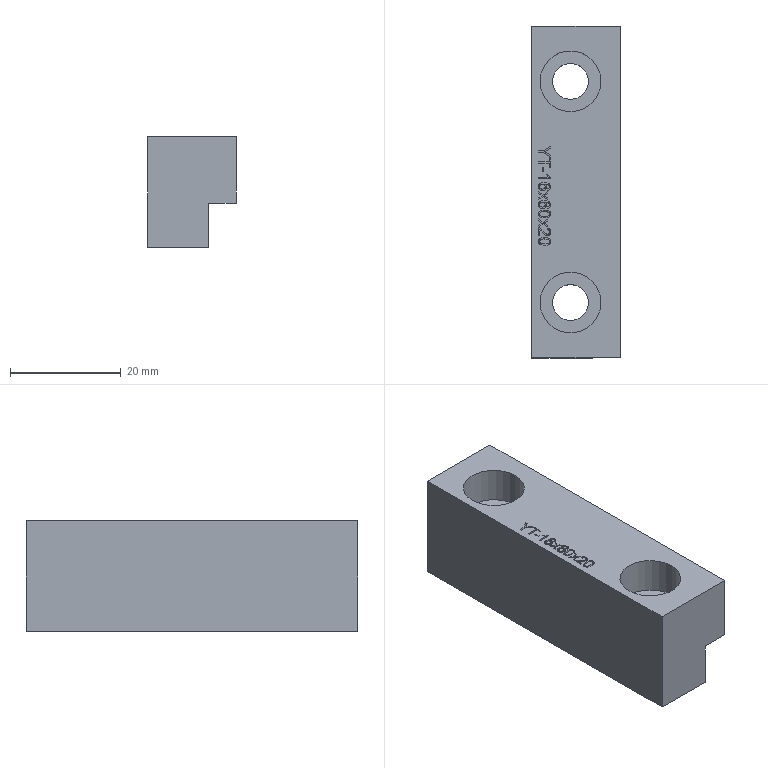Part | STEP file | lll_id302_x_t | 1 solid | 161 faces | box 16 x 60 x 20 mm | volume 14663 mm3 | plane 83 | other 74 | cylinder 4 | commonest cylinder face diameters 6.5 x2 11 x2